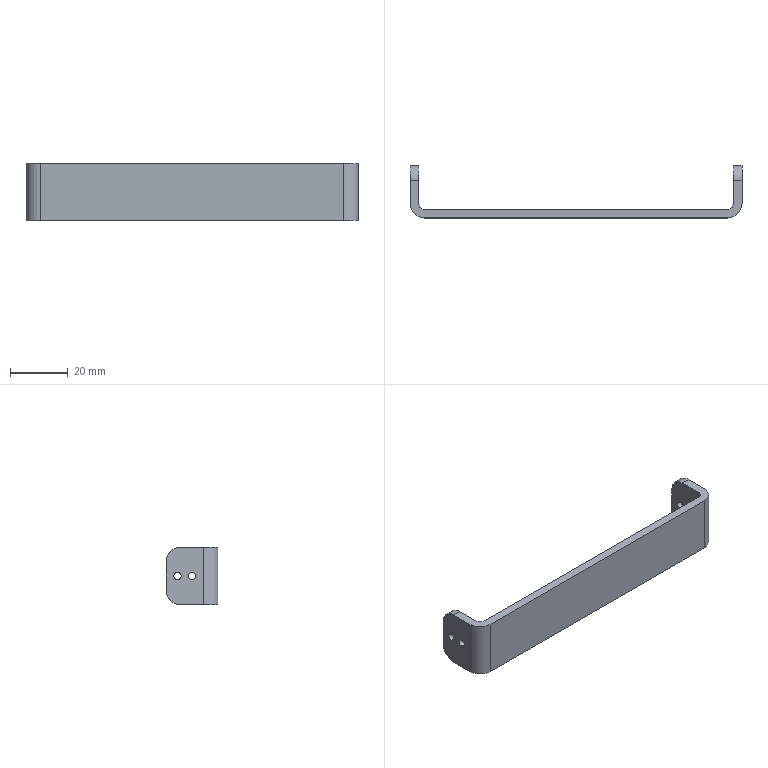Part | SolidWorks | features Fillet 3, Extrusion 1, HoleWzd 1, ICE 1 | 1 solid | 26 faces | box 115 x 18 x 20 mm | volume 8396 mm3 | cylinder 16 | plane 10 | commonest cylinder face diameters 2.5 x8 10 x6 4 x2
STEP:
#1=CARTESIAN_POINT('',(-54.5,14.,-1.25));
#2=VERTEX_POINT('',#1);
#3=CARTESIAN_POINT('',(-54.5,14.,1.25));
#4=VERTEX_POINT('',#3);
#5=CARTESIAN_POINT('',(-54.5,14.,0.));
#6=DIRECTION('',(-1.,0.,0.));
#7=DIRECTION('',(0.,0.,1.));
#8=AXIS2_PLACEMENT_3D('',#5,#6,#7);
#9=CIRCLE('',#8,1.25);
#10=EDGE_CURVE('',#2,#4,#9,.T.);
#11=ORIENTED_EDGE('',*,*,#10,.F.);
#12=CARTESIAN_POINT('',(-57.5,14.,-1.25));
#13=VERTEX_POINT('',#12);
#14=CARTESIAN_POINT('',(-57.5,14.,-1.25));
#15=DIRECTION('',(-1.,0.,0.));
#16=VECTOR('',#15,1000.);
#17=LINE('',#14,#16);
#18=EDGE_CURVE('',#2,#13,#17,.T.);
#19=ORIENTED_EDGE('',*,*,#18,.T.);
#20=CARTESIAN_POINT('',(-57.5,14.,1.25));
#21=VERTEX_POINT('',#20);
#22=CARTESIAN_POINT('',(-57.5,14.,0.));
#23=DIRECTION('',(-1.,0.,0.));
#24=DIRECTION('',(0.,0.,1.));
#25=AXIS2_PLACEMENT_3D('',#22,#23,#24);
#26=CIRCLE('',#25,1.25);
#27=EDGE_CURVE('',#13,#21,#26,.T.);
#28=ORIENTED_EDGE('',*,*,#27,.T.);
#29=CARTESIAN_POINT('',(-57.5,14.,1.25));
#30=DIRECTION('',(-1.,0.,0.));
#31=VECTOR('',#30,1000.);
#32=LINE('',#29,#31);
#33=EDGE_CURVE('',#4,#21,#32,.T.);
#34=ORIENTED_EDGE('',*,*,#33,.F.);
#35=EDGE_LOOP('',(#11,#19,#28,#34));
#36=FACE_OUTER_BOUND('',#35,.T.);
#37=CARTESIAN_POINT('',(-57.5,14.,0.));
#38=DIRECTION('',(-1.,0.,0.));
#39=DIRECTION('',(0.,0.,1.));
#40=AXIS2_PLACEMENT_3D('',#37,#38,#39);
#41=CYLINDRICAL_SURFACE('',#40,1.25);
#42=ADVANCED_FACE('',(#36),#41,.F.);
#43=CARTESIAN_POINT('',(57.5,14.,-1.25));
#44=VERTEX_POINT('',#43);
#45=CARTESIAN_POINT('',(57.5,14.,1.25));
#46=VERTEX_POINT('',#45);
#47=CARTESIAN_POINT('',(57.5,14.,0.));
#48=DIRECTION('',(-1.,0.,0.));
#49=DIRECTION('',(0.,0.,1.));
#50=AXIS2_PLACEMENT_3D('',#47,#48,#49);
#51=CIRCLE('',#50,1.25);
#52=EDGE_CURVE('',#44,#46,#51,.T.);
#53=ORIENTED_EDGE('',*,*,#52,.F.);
#54=CARTESIAN_POINT('',(54.5,14.,-1.25));
#55=VERTEX_POINT('',#54);
#56=CARTESIAN_POINT('',(-57.5,14.,-1.25));
#57=DIRECTION('',(-1.,0.,0.));
#58=VECTOR('',#57,1000.);
#59=LINE('',#56,#58);
#60=EDGE_CURVE('',#44,#55,#59,.T.);
#61=ORIENTED_EDGE('',*,*,#60,.T.);
#62=CARTESIAN_POINT('',(54.5,14.,1.25));
#63=VERTEX_POINT('',#62);
#64=CARTESIAN_POINT('',(54.5,14.,0.));
#65=DIRECTION('',(1.,0.,0.));
#66=DIRECTION('',(0.,0.,-1.));
#67=AXIS2_PLACEMENT_3D('',#64,#65,#66);
#68=CIRCLE('',#67,1.25);
#69=EDGE_CURVE('',#63,#55,#68,.T.);
#70=ORIENTED_EDGE('',*,*,#69,.F.);
#71=CARTESIAN_POINT('',(-57.5,14.,1.25));
#72=DIRECTION('',(-1.,0.,0.));
#73=VECTOR('',#72,1000.);
#74=LINE('',#71,#73);
#75=EDGE_CURVE('',#46,#63,#74,.T.);
#76=ORIENTED_EDGE('',*,*,#75,.F.);
#77=EDGE_LOOP('',(#53,#61,#70,#76));
#78=FACE_OUTER_BOUND('',#77,.T.);
#79=CARTESIAN_POINT('',(-57.5,14.,0.));
#80=DIRECTION('',(-1.,0.,0.));
#81=DIRECTION('',(0.,0.,1.));
#82=AXIS2_PLACEMENT_3D('',#79,#80,#81);
#83=CYLINDRICAL_SURFACE('',#82,1.25);
#84=ADVANCED_FACE('',(#78),#83,.F.);
#85=CARTESIAN_POINT('',(-54.5,9.,-1.25));
#86=VERTEX_POINT('',#85);
#87=CARTESIAN_POINT('',(-54.5,9.,1.25));
#88=VERTEX_POINT('',#87);
#89=CARTESIAN_POINT('',(-54.5,9.,0.));
#90=DIRECTION('',(-1.,0.,0.));
#91=DIRECTION('',(0.,0.,1.));
#92=AXIS2_PLACEMENT_3D('',#89,#90,#91);
#93=CIRCLE('',#92,1.25);
#94=EDGE_CURVE('',#86,#88,#93,.T.);
#95=ORIENTED_EDGE('',*,*,#94,.F.);
#96=CARTESIAN_POINT('',(-57.5,9.,-1.25));
#97=VERTEX_POINT('',#96);
#98=CARTESIAN_POINT('',(-57.5,9.,-1.25));
#99=DIRECTION('',(-1.,0.,0.));
#100=VECTOR('',#99,1000.);
#101=LINE('',#98,#100);
#102=EDGE_CURVE('',#86,#97,#101,.T.);
#103=ORIENTED_EDGE('',*,*,#102,.T.);
#104=CARTESIAN_POINT('',(-57.5,9.,1.25));
#105=VERTEX_POINT('',#104);
#106=CARTESIAN_POINT('',(-57.5,9.,0.));
#107=DIRECTION('',(-1.,0.,0.));
#108=DIRECTION('',(0.,0.,1.));
#109=AXIS2_PLACEMENT_3D('',#106,#107,#108);
#110=CIRCLE('',#109,1.25);
#111=EDGE_CURVE('',#97,#105,#110,.T.);
#112=ORIENTED_EDGE('',*,*,#111,.T.);
#113=CARTESIAN_POINT('',(-57.5,9.,1.25));
#114=DIRECTION('',(-1.,0.,0.));
#115=VECTOR('',#114,1000.);
#116=LINE('',#113,#115);
#117=EDGE_CURVE('',#88,#105,#116,.T.);
#118=ORIENTED_EDGE('',*,*,#117,.F.);
#119=EDGE_LOOP('',(#95,#103,#112,#118));
#120=FACE_OUTER_BOUND('',#119,.T.);
#121=CARTESIAN_POINT('',(-57.5,9.,0.));
#122=DIRECTION('',(-1.,0.,0.));
#123=DIRECTION('',(0.,0.,1.));
#124=AXIS2_PLACEMENT_3D('',#121,#122,#123);
#125=CYLINDRICAL_SURFACE('',#124,1.25);
#126=ADVANCED_FACE('',(#120),#125,.F.);
#127=CARTESIAN_POINT('',(57.5,9.,-1.25));
#128=VERTEX_POINT('',#127);
#129=CARTESIAN_POINT('',(57.5,9.,1.25));
#130=VERTEX_POINT('',#129);
#131=CARTESIAN_POINT('',(57.5,9.,0.));
#132=DIRECTION('',(-1.,0.,0.));
#133=DIRECTION('',(0.,0.,1.));
#134=AXIS2_PLACEMENT_3D('',#131,#132,#133);
#135=CIRCLE('',#134,1.25);
#136=EDGE_CURVE('',#128,#130,#135,.T.);
#137=ORIENTED_EDGE('',*,*,#136,.F.);
#138=CARTESIAN_POINT('',(54.5,9.,-1.25));
#139=VERTEX_POINT('',#138);
#140=CARTESIAN_POINT('',(-57.5,9.,-1.25));
#141=DIRECTION('',(-1.,0.,0.));
#142=VECTOR('',#141,1000.);
#143=LINE('',#140,#142);
#144=EDGE_CURVE('',#128,#139,#143,.T.);
#145=ORIENTED_EDGE('',*,*,#144,.T.);
#146=CARTESIAN_POINT('',(54.5,9.,1.25));
#147=VERTEX_POINT('',#146);
#148=CARTESIAN_POINT('',(54.5,9.,0.));
#149=DIRECTION('',(1.,0.,0.));
#150=DIRECTION('',(0.,0.,-1.));
#151=AXIS2_PLACEMENT_3D('',#148,#149,#150);
#152=CIRCLE('',#151,1.25);
#153=EDGE_CURVE('',#147,#139,#152,.T.);
#154=ORIENTED_EDGE('',*,*,#153,.F.);
#155=CARTESIAN_POINT('',(-57.5,9.,1.25));
#156=DIRECTION('',(-1.,0.,0.));
#157=VECTOR('',#156,1000.);
#158=LINE('',#155,#157);
#159=EDGE_CURVE('',#130,#147,#158,.T.);
#160=ORIENTED_EDGE('',*,*,#159,.F.);
#161=EDGE_LOOP('',(#137,#145,#154,#160));
#162=FACE_OUTER_BOUND('',#161,.T.);
#163=CARTESIAN_POINT('',(-57.5,9.,0.));
#164=DIRECTION('',(-1.,0.,0.));
#165=DIRECTION('',(0.,0.,1.));
#166=AXIS2_PLACEMENT_3D('',#163,#164,#165);
#167=CYLINDRICAL_SURFACE('',#166,1.25);
#168=ADVANCED_FACE('',(#162),#167,.F.);
#169=CARTESIAN_POINT('',(-57.5,9.,0.));
#170=DIRECTION('',(-1.,0.,0.));
#171=DIRECTION('',(0.,0.,1.));
#172=AXIS2_PLACEMENT_3D('',#169,#170,#171);
#173=CIRCLE('',#172,1.25);
#174=EDGE_CURVE('',#105,#97,#173,.T.);
#175=ORIENTED_EDGE('',*,*,#174,.F.);
#176=ORIENTED_EDGE('',*,*,#111,.F.);
#177=EDGE_LOOP('',(#175,#176));
#178=FACE_BOUND('',#177,.T.);
#179=CARTESIAN_POINT('',(-57.5,13.,10.));
#180=VERTEX_POINT('',#179);
#181=CARTESIAN_POINT('',(-57.5,5.,10.));
#182=VERTEX_POINT('',#181);
#183=CARTESIAN_POINT('',(-57.5,3.,10.));
#184=DIRECTION('',(0.,-1.,0.));
#185=VECTOR('',#184,1000.);
#186=LINE('',#183,#185);
#187=EDGE_CURVE('',#180,#182,#186,.T.);
#188=ORIENTED_EDGE('',*,*,#187,.F.);
#189=CARTESIAN_POINT('',(-57.5,18.,5.));
#190=VERTEX_POINT('',#189);
#191=CARTESIAN_POINT('',(-57.5,13.,5.));
#192=DIRECTION('',(-1.,0.,0.));
#193=DIRECTION('',(0.,0.,-1.));
#194=AXIS2_PLACEMENT_3D('',#191,#192,#193);
#195=CIRCLE('',#194,5.);
#196=EDGE_CURVE('',#180,#190,#195,.T.);
#197=ORIENTED_EDGE('',*,*,#196,.T.);
#198=CARTESIAN_POINT('',(-57.5,18.,-5.));
#199=VERTEX_POINT('',#198);
#200=CARTESIAN_POINT('',(-57.5,18.,-10.));
#201=DIRECTION('',(0.,0.,1.));
#202=VECTOR('',#201,1000.);
#203=LINE('',#200,#202);
#204=EDGE_CURVE('',#199,#190,#203,.T.);
#205=ORIENTED_EDGE('',*,*,#204,.F.);
#206=CARTESIAN_POINT('',(-57.5,13.,-10.));
#207=VERTEX_POINT('',#206);
#208=CARTESIAN_POINT('',(-57.5,13.,-5.));
#209=DIRECTION('',(-1.,0.,0.));
#210=DIRECTION('',(0.,0.,-1.));
#211=AXIS2_PLACEMENT_3D('',#208,#209,#210);
#212=CIRCLE('',#211,5.);
#213=EDGE_CURVE('',#199,#207,#212,.T.);
#214=ORIENTED_EDGE('',*,*,#213,.T.);
#215=CARTESIAN_POINT('',(-57.5,5.,-10.));
#216=VERTEX_POINT('',#215);
#217=CARTESIAN_POINT('',(-57.5,3.,-10.));
#218=DIRECTION('',(0.,-1.,0.));
#219=VECTOR('',#218,1000.);
#220=LINE('',#217,#219);
#221=EDGE_CURVE('',#207,#216,#220,.T.);
#222=ORIENTED_EDGE('',*,*,#221,.T.);
#223=CARTESIAN_POINT('',(-57.5,5.,10.));
#224=DIRECTION('',(0.,0.,1.));
#225=VECTOR('',#224,1000.);
#226=LINE('',#223,#225);
#227=EDGE_CURVE('',#216,#182,#226,.T.);
#228=ORIENTED_EDGE('',*,*,#227,.T.);
#229=EDGE_LOOP('',(#188,#197,#205,#214,#222,#228));
#230=FACE_OUTER_BOUND('',#229,.T.);
#231=CARTESIAN_POINT('',(-57.5,14.,0.));
#232=DIRECTION('',(-1.,0.,0.));
#233=DIRECTION('',(0.,0.,1.));
#234=AXIS2_PLACEMENT_3D('',#231,#232,#233);
#235=CIRCLE('',#234,1.25);
#236=EDGE_CURVE('',#21,#13,#235,.T.);
#237=ORIENTED_EDGE('',*,*,#236,.F.);
#238=ORIENTED_EDGE('',*,*,#27,.F.);
#239=EDGE_LOOP('',(#237,#238));
#240=FACE_BOUND('',#239,.T.);
#241=CARTESIAN_POINT('',(-57.5,3.,10.));
#242=DIRECTION('',(1.,0.,0.));
#243=DIRECTION('',(0.,0.,-1.));
#244=AXIS2_PLACEMENT_3D('',#241,#242,#243);
#245=PLANE('',#244);
#246=ADVANCED_FACE('',(#178,#230,#240),#245,.F.);
#247=CARTESIAN_POINT('',(-52.5,3.,10.));
#248=VERTEX_POINT('',#247);
#249=CARTESIAN_POINT('',(52.5,3.,10.));
#250=VERTEX_POINT('',#249);
#251=CARTESIAN_POINT('',(-57.5,3.,10.));
#252=DIRECTION('',(1.,0.,0.));
#253=VECTOR('',#252,1000.);
#254=LINE('',#251,#253);
#255=EDGE_CURVE('',#248,#250,#254,.T.);
#256=ORIENTED_EDGE('',*,*,#255,.T.);
#257=CARTESIAN_POINT('',(52.5,3.,-10.));
#258=VERTEX_POINT('',#257);
#259=CARTESIAN_POINT('',(52.5,3.,-10.));
#260=DIRECTION('',(0.,0.,-1.));
#261=VECTOR('',#260,1000.);
#262=LINE('',#259,#261);
#263=EDGE_CURVE('',#250,#258,#262,.T.);
#264=ORIENTED_EDGE('',*,*,#263,.T.);
#265=CARTESIAN_POINT('',(-52.5,3.,-10.));
#266=VERTEX_POINT('',#265);
#267=CARTESIAN_POINT('',(-57.5,3.,-10.));
#268=DIRECTION('',(-1.,0.,0.));
#269=VECTOR('',#268,1000.);
#270=LINE('',#267,#269);
#271=EDGE_CURVE('',#258,#266,#270,.T.);
#272=ORIENTED_EDGE('',*,*,#271,.T.);
#273=CARTESIAN_POINT('',(-52.5,3.,10.));
#274=DIRECTION('',(0.,0.,1.));
#275=VECTOR('',#274,1000.);
#276=LINE('',#273,#275);
#277=EDGE_CURVE('',#266,#248,#276,.T.);
#278=ORIENTED_EDGE('',*,*,#277,.T.);
#279=EDGE_LOOP('',(#256,#264,#272,#278));
#280=FACE_OUTER_BOUND('',#279,.T.);
#281=CARTESIAN_POINT('',(0.,3.,0.));
#282=DIRECTION('',(0.,-1.,0.));
#283=DIRECTION('',(0.,0.,-1.));
#284=AXIS2_PLACEMENT_3D('',#281,#282,#283);
#285=PLANE('',#284);
#286=ADVANCED_FACE('',(#280),#285,.F.);
#287=CARTESIAN_POINT('',(57.5,14.,0.));
#288=DIRECTION('',(-1.,0.,0.));
#289=DIRECTION('',(0.,0.,1.));
#290=AXIS2_PLACEMENT_3D('',#287,#288,#289);
#291=CIRCLE('',#290,1.25);
#292=EDGE_CURVE('',#46,#44,#291,.T.);
#293=ORIENTED_EDGE('',*,*,#292,.T.);
#294=ORIENTED_EDGE('',*,*,#52,.T.);
#295=EDGE_LOOP('',(#293,#294));
#296=FACE_BOUND('',#295,.T.);
#297=CARTESIAN_POINT('',(57.5,9.,0.));
#298=DIRECTION('',(-1.,0.,0.));
#299=DIRECTION('',(0.,0.,1.));
#300=AXIS2_PLACEMENT_3D('',#297,#298,#299);
#301=CIRCLE('',#300,1.25);
#302=EDGE_CURVE('',#130,#128,#301,.T.);
#303=ORIENTED_EDGE('',*,*,#302,.T.);
#304=ORIENTED_EDGE('',*,*,#136,.T.);
#305=EDGE_LOOP('',(#303,#304));
#306=FACE_BOUND('',#305,.T.);
#307=CARTESIAN_POINT('',(57.5,18.,5.));
#308=VERTEX_POINT('',#307);
#309=CARTESIAN_POINT('',(57.5,18.,-5.));
#310=VERTEX_POINT('',#309);
#311=CARTESIAN_POINT('',(57.5,18.,-10.));
#312=DIRECTION('',(0.,0.,-1.));
#313=VECTOR('',#312,1000.);
#314=LINE('',#311,#313);
#315=EDGE_CURVE('',#308,#310,#314,.T.);
#316=ORIENTED_EDGE('',*,*,#315,.F.);
#317=CARTESIAN_POINT('',(57.5,13.,10.));
#318=VERTEX_POINT('',#317);
#319=CARTESIAN_POINT('',(57.5,13.,5.));
#320=DIRECTION('',(1.,0.,0.));
#321=DIRECTION('',(0.,0.,1.));
#322=AXIS2_PLACEMENT_3D('',#319,#320,#321);
#323=CIRCLE('',#322,5.);
#324=EDGE_CURVE('',#308,#318,#323,.T.);
#325=ORIENTED_EDGE('',*,*,#324,.T.);
#326=CARTESIAN_POINT('',(57.5,5.,10.));
#327=VERTEX_POINT('',#326);
#328=CARTESIAN_POINT('',(57.5,3.,10.));
#329=DIRECTION('',(0.,-1.,0.));
#330=VECTOR('',#329,1000.);
#331=LINE('',#328,#330);
#332=EDGE_CURVE('',#318,#327,#331,.T.);
#333=ORIENTED_EDGE('',*,*,#332,.T.);
#334=CARTESIAN_POINT('',(57.5,5.,-10.));
#335=VERTEX_POINT('',#334);
#336=CARTESIAN_POINT('',(57.5,5.,-10.));
#337=DIRECTION('',(0.,0.,-1.));
#338=VECTOR('',#337,1000.);
#339=LINE('',#336,#338);
#340=EDGE_CURVE('',#327,#335,#339,.T.);
#341=ORIENTED_EDGE('',*,*,#340,.T.);
#342=CARTESIAN_POINT('',(57.5,13.,-10.));
#343=VERTEX_POINT('',#342);
#344=CARTESIAN_POINT('',(57.5,3.,-10.));
#345=DIRECTION('',(0.,-1.,0.));
#346=VECTOR('',#345,1000.);
#347=LINE('',#344,#346);
#348=EDGE_CURVE('',#343,#335,#347,.T.);
#349=ORIENTED_EDGE('',*,*,#348,.F.);
#350=CARTESIAN_POINT('',(57.5,13.,-5.));
#351=DIRECTION('',(1.,0.,0.));
#352=DIRECTION('',(0.,0.,1.));
#353=AXIS2_PLACEMENT_3D('',#350,#351,#352);
#354=CIRCLE('',#353,5.);
#355=EDGE_CURVE('',#343,#310,#354,.T.);
#356=ORIENTED_EDGE('',*,*,#355,.T.);
#357=EDGE_LOOP('',(#316,#325,#333,#341,#349,#356));
#358=FACE_OUTER_BOUND('',#357,.T.);
#359=CARTESIAN_POINT('',(57.5,3.,10.));
#360=DIRECTION('',(-1.,0.,0.));
#361=DIRECTION('',(0.,0.,1.));
#362=AXIS2_PLACEMENT_3D('',#359,#360,#361);
#363=PLANE('',#362);
#364=ADVANCED_FACE('',(#296,#306,#358),#363,.F.);
#365=ORIENTED_EDGE('',*,*,#221,.F.);
#366=CARTESIAN_POINT('',(-54.5,13.,-10.));
#367=VERTEX_POINT('',#366);
#368=CARTESIAN_POINT('',(-54.5,13.,-10.));
#369=DIRECTION('',(1.,0.,0.));
#370=VECTOR('',#369,1000.);
#371=LINE('',#368,#370);
#372=EDGE_CURVE('',#207,#367,#371,.T.);
#373=ORIENTED_EDGE('',*,*,#372,.T.);
#374=CARTESIAN_POINT('',(-54.5,5.,-10.));
#375=VERTEX_POINT('',#374);
#376=CARTESIAN_POINT('',(-54.5,18.,-10.));
#377=DIRECTION('',(0.,-1.,0.));
#378=VECTOR('',#377,1000.);
#379=LINE('',#376,#378);
#380=EDGE_CURVE('',#367,#375,#379,.T.);
#381=ORIENTED_EDGE('',*,*,#380,.T.);
#382=CARTESIAN_POINT('',(-52.5,5.,-10.));
#383=DIRECTION('',(0.,0.,1.));
#384=DIRECTION('',(1.,0.,0.));
#385=AXIS2_PLACEMENT_3D('',#382,#383,#384);
#386=CIRCLE('',#385,2.);
#387=EDGE_CURVE('',#375,#266,#386,.T.);
#388=ORIENTED_EDGE('',*,*,#387,.T.);
#389=ORIENTED_EDGE('',*,*,#271,.F.);
#390=CARTESIAN_POINT('',(54.5,5.,-10.));
#391=VERTEX_POINT('',#390);
#392=CARTESIAN_POINT('',(52.5,5.,-10.));
#393=DIRECTION('',(0.,0.,1.));
#394=DIRECTION('',(1.,0.,0.));
#395=AXIS2_PLACEMENT_3D('',#392,#393,#394);
#396=CIRCLE('',#395,2.);
#397=EDGE_CURVE('',#258,#391,#396,.T.);
#398=ORIENTED_EDGE('',*,*,#397,.T.);
#399=CARTESIAN_POINT('',(54.5,13.,-10.));
#400=VERTEX_POINT('',#399);
#401=CARTESIAN_POINT('',(54.5,18.,-10.));
#402=DIRECTION('',(0.,-1.,0.));
#403=VECTOR('',#402,1000.);
#404=LINE('',#401,#403);
#405=EDGE_CURVE('',#400,#391,#404,.T.);
#406=ORIENTED_EDGE('',*,*,#405,.F.);
#407=CARTESIAN_POINT('',(-57.5,13.,-10.));
#408=DIRECTION('',(1.,0.,0.));
#409=VECTOR('',#408,1000.);
#410=LINE('',#407,#409);
#411=EDGE_CURVE('',#400,#343,#410,.T.);
#412=ORIENTED_EDGE('',*,*,#411,.T.);
#413=ORIENTED_EDGE('',*,*,#348,.T.);
#414=CARTESIAN_POINT('',(52.5,0.,-10.));
#415=VERTEX_POINT('',#414);
#416=CARTESIAN_POINT('',(52.5,5.,-10.));
#417=DIRECTION('',(0.,0.,-1.));
#418=DIRECTION('',(1.,0.,0.));
#419=AXIS2_PLACEMENT_3D('',#416,#417,#418);
#420=CIRCLE('',#419,5.);
#421=EDGE_CURVE('',#335,#415,#420,.T.);
#422=ORIENTED_EDGE('',*,*,#421,.T.);
#423=CARTESIAN_POINT('',(-52.5,0.,-10.));
#424=VERTEX_POINT('',#423);
#425=CARTESIAN_POINT('',(-57.5,0.,-10.));
#426=DIRECTION('',(-1.,0.,0.));
#427=VECTOR('',#426,1000.);
#428=LINE('',#425,#427);
#429=EDGE_CURVE('',#415,#424,#428,.T.);
#430=ORIENTED_EDGE('',*,*,#429,.T.);
#431=CARTESIAN_POINT('',(-52.5,5.,-10.));
#432=DIRECTION('',(0.,0.,-1.));
#433=DIRECTION('',(1.,0.,0.));
#434=AXIS2_PLACEMENT_3D('',#431,#432,#433);
#435=CIRCLE('',#434,5.);
#436=EDGE_CURVE('',#424,#216,#435,.T.);
#437=ORIENTED_EDGE('',*,*,#436,.T.);
#438=EDGE_LOOP('',(#365,#373,#381,#388,#389,#398,#406,#412,#413,#422,#430,#437));
#439=FACE_OUTER_BOUND('',#438,.T.);
#440=CARTESIAN_POINT('',(-57.5,3.,-10.));
#441=DIRECTION('',(0.,0.,1.));
#442=DIRECTION('',(1.,0.,0.));
#443=AXIS2_PLACEMENT_3D('',#440,#441,#442);
#444=PLANE('',#443);
#445=ADVANCED_FACE('',(#439),#444,.F.);
#446=CARTESIAN_POINT('',(-54.5,13.,10.));
#447=VERTEX_POINT('',#446);
#448=CARTESIAN_POINT('',(-54.5,5.,10.));
#449=VERTEX_POINT('',#448);
#450=CARTESIAN_POINT('',(-54.5,18.,10.));
#451=DIRECTION('',(0.,-1.,0.));
#452=VECTOR('',#451,1000.);
#453=LINE('',#450,#452);
#454=EDGE_CURVE('',#447,#449,#453,.T.);
#455=ORIENTED_EDGE('',*,*,#454,.F.);
#456=CARTESIAN_POINT('',(-57.5,13.,10.));
#457=DIRECTION('',(-1.,0.,0.));
#458=VECTOR('',#457,1000.);
#459=LINE('',#456,#458);
#460=EDGE_CURVE('',#447,#180,#459,.T.);
#461=ORIENTED_EDGE('',*,*,#460,.T.);
#462=ORIENTED_EDGE('',*,*,#187,.T.);
#463=CARTESIAN_POINT('',(-52.5,0.,10.));
#464=VERTEX_POINT('',#463);
#465=CARTESIAN_POINT('',(-52.5,5.,10.));
#466=DIRECTION('',(0.,0.,1.));
#467=DIRECTION('',(-1.,0.,0.));
#468=AXIS2_PLACEMENT_3D('',#465,#466,#467);
#469=CIRCLE('',#468,5.);
#470=EDGE_CURVE('',#182,#464,#469,.T.);
#471=ORIENTED_EDGE('',*,*,#470,.T.);
#472=CARTESIAN_POINT('',(52.5,0.,10.));
#473=VERTEX_POINT('',#472);
#474=CARTESIAN_POINT('',(-57.5,0.,10.));
#475=DIRECTION('',(1.,0.,0.));
#476=VECTOR('',#475,1000.);
#477=LINE('',#474,#476);
#478=EDGE_CURVE('',#464,#473,#477,.T.);
#479=ORIENTED_EDGE('',*,*,#478,.T.);
#480=CARTESIAN_POINT('',(52.5,5.,10.));
#481=DIRECTION('',(0.,0.,1.));
#482=DIRECTION('',(-1.,0.,0.));
#483=AXIS2_PLACEMENT_3D('',#480,#481,#482);
#484=CIRCLE('',#483,5.);
#485=EDGE_CURVE('',#473,#327,#484,.T.);
#486=ORIENTED_EDGE('',*,*,#485,.T.);
#487=ORIENTED_EDGE('',*,*,#332,.F.);
#488=CARTESIAN_POINT('',(54.5,13.,10.));
#489=VERTEX_POINT('',#488);
#490=CARTESIAN_POINT('',(-57.5,13.,10.));
#491=DIRECTION('',(-1.,0.,0.));
#492=VECTOR('',#491,1000.);
#493=LINE('',#490,#492);
#494=EDGE_CURVE('',#318,#489,#493,.T.);
#495=ORIENTED_EDGE('',*,*,#494,.T.);
#496=CARTESIAN_POINT('',(54.5,5.,10.));
#497=VERTEX_POINT('',#496);
#498=CARTESIAN_POINT('',(54.5,18.,10.));
#499=DIRECTION('',(0.,-1.,0.));
#500=VECTOR('',#499,1000.);
#501=LINE('',#498,#500);
#502=EDGE_CURVE('',#489,#497,#501,.T.);
#503=ORIENTED_EDGE('',*,*,#502,.T.);
#504=CARTESIAN_POINT('',(52.5,5.,10.));
#505=DIRECTION('',(0.,0.,-1.));
#506=DIRECTION('',(-1.,0.,0.));
#507=AXIS2_PLACEMENT_3D('',#504,#505,#506);
#508=CIRCLE('',#507,2.);
#509=EDGE_CURVE('',#497,#250,#508,.T.);
#510=ORIENTED_EDGE('',*,*,#509,.T.);
#511=ORIENTED_EDGE('',*,*,#255,.F.);
#512=CARTESIAN_POINT('',(-52.5,5.,10.));
#513=DIRECTION('',(0.,0.,-1.));
#514=DIRECTION('',(-1.,0.,0.));
#515=AXIS2_PLACEMENT_3D('',#512,#513,#514);
#516=CIRCLE('',#515,2.);
#517=EDGE_CURVE('',#248,#449,#516,.T.);
#518=ORIENTED_EDGE('',*,*,#517,.T.);
#519=EDGE_LOOP('',(#455,#461,#462,#471,#479,#486,#487,#495,#503,#510,#511,#518));
#520=FACE_OUTER_BOUND('',#519,.T.);
#521=CARTESIAN_POINT('',(-57.5,3.,10.));
#522=DIRECTION('',(0.,0.,-1.));
#523=DIRECTION('',(-1.,0.,0.));
#524=AXIS2_PLACEMENT_3D('',#521,#522,#523);
#525=PLANE('',#524);
#526=ADVANCED_FACE('',(#520),#525,.F.);
#527=ORIENTED_EDGE('',*,*,#429,.F.);
#528=CARTESIAN_POINT('',(52.5,0.,10.));
#529=DIRECTION('',(0.,0.,1.));
#530=VECTOR('',#529,1000.);
#531=LINE('',#528,#530);
#532=EDGE_CURVE('',#415,#473,#531,.T.);
#533=ORIENTED_EDGE('',*,*,#532,.T.);
#534=ORIENTED_EDGE('',*,*,#478,.F.);
#535=CARTESIAN_POINT('',(-52.5,0.,-10.));
#536=DIRECTION('',(0.,0.,-1.));
#537=VECTOR('',#536,1000.);
#538=LINE('',#535,#537);
#539=EDGE_CURVE('',#464,#424,#538,.T.);
#540=ORIENTED_EDGE('',*,*,#539,.T.);
#541=EDGE_LOOP('',(#527,#533,#534,#540));
#542=FACE_OUTER_BOUND('',#541,.T.);
#543=CARTESIAN_POINT('',(0.,0.,0.));
#544=DIRECTION('',(0.,-1.,0.));
#545=DIRECTION('',(0.,0.,-1.));
#546=AXIS2_PLACEMENT_3D('',#543,#544,#545);
#547=PLANE('',#546);
#548=ADVANCED_FACE('',(#542),#547,.T.);
#549=CARTESIAN_POINT('',(-54.5,14.,0.));
#550=DIRECTION('',(-1.,0.,0.));
#551=DIRECTION('',(0.,0.,1.));
#552=AXIS2_PLACEMENT_3D('',#549,#550,#551);
#553=CIRCLE('',#552,1.25);
#554=EDGE_CURVE('',#4,#2,#553,.T.);
#555=ORIENTED_EDGE('',*,*,#554,.T.);
#556=ORIENTED_EDGE('',*,*,#10,.T.);
#557=EDGE_LOOP('',(#555,#556));
#558=FACE_BOUND('',#557,.T.);
#559=CARTESIAN_POINT('',(-54.5,9.,0.));
#560=DIRECTION('',(-1.,0.,0.));
#561=DIRECTION('',(0.,0.,1.));
#562=AXIS2_PLACEMENT_3D('',#559,#560,#561);
#563=CIRCLE('',#562,1.25);
#564=EDGE_CURVE('',#88,#86,#563,.T.);
#565=ORIENTED_EDGE('',*,*,#564,.T.);
#566=ORIENTED_EDGE('',*,*,#94,.T.);
#567=EDGE_LOOP('',(#565,#566));
#568=FACE_BOUND('',#567,.T.);
#569=CARTESIAN_POINT('',(-54.5,18.,5.));
#570=VERTEX_POINT('',#569);
#571=CARTESIAN_POINT('',(-54.5,18.,-5.));
#572=VERTEX_POINT('',#571);
#573=CARTESIAN_POINT('',(-54.5,18.,-10.));
#574=DIRECTION('',(0.,0.,-1.));
#575=VECTOR('',#574,1000.);
#576=LINE('',#573,#575);
#577=EDGE_CURVE('',#570,#572,#576,.T.);
#578=ORIENTED_EDGE('',*,*,#577,.F.);
#579=CARTESIAN_POINT('',(-54.5,13.,5.));
#580=DIRECTION('',(1.,0.,0.));
#581=DIRECTION('',(0.,0.,1.));
#582=AXIS2_PLACEMENT_3D('',#579,#580,#581);
#583=CIRCLE('',#582,5.);
#584=EDGE_CURVE('',#570,#447,#583,.T.);
#585=ORIENTED_EDGE('',*,*,#584,.T.);
#586=ORIENTED_EDGE('',*,*,#454,.T.);
#587=CARTESIAN_POINT('',(-54.5,5.,-10.));
#588=DIRECTION('',(0.,0.,-1.));
#589=VECTOR('',#588,1000.);
#590=LINE('',#587,#589);
#591=EDGE_CURVE('',#449,#375,#590,.T.);
#592=ORIENTED_EDGE('',*,*,#591,.T.);
#593=ORIENTED_EDGE('',*,*,#380,.F.);
#594=CARTESIAN_POINT('',(-54.5,13.,-5.));
#595=DIRECTION('',(1.,0.,0.));
#596=DIRECTION('',(0.,0.,1.));
#597=AXIS2_PLACEMENT_3D('',#594,#595,#596);
#598=CIRCLE('',#597,5.);
#599=EDGE_CURVE('',#367,#572,#598,.T.);
#600=ORIENTED_EDGE('',*,*,#599,.T.);
#601=EDGE_LOOP('',(#578,#585,#586,#592,#593,#600));
#602=FACE_OUTER_BOUND('',#601,.T.);
#603=CARTESIAN_POINT('',(-54.5,18.,-10.));
#604=DIRECTION('',(-1.,0.,0.));
#605=DIRECTION('',(0.,0.,1.));
#606=AXIS2_PLACEMENT_3D('',#603,#604,#605);
#607=PLANE('',#606);
#608=ADVANCED_FACE('',(#558,#568,#602),#607,.F.);
#609=ORIENTED_EDGE('',*,*,#204,.T.);
#610=CARTESIAN_POINT('',(-54.5,18.,5.));
#611=DIRECTION('',(1.,0.,0.));
#612=VECTOR('',#611,1000.);
#613=LINE('',#610,#612);
#614=EDGE_CURVE('',#190,#570,#613,.T.);
#615=ORIENTED_EDGE('',*,*,#614,.T.);
#616=ORIENTED_EDGE('',*,*,#577,.T.);
#617=CARTESIAN_POINT('',(-57.5,18.,-5.));
#618=DIRECTION('',(-1.,0.,0.));
#619=VECTOR('',#618,1000.);
#620=LINE('',#617,#619);
#621=EDGE_CURVE('',#572,#199,#620,.T.);
#622=ORIENTED_EDGE('',*,*,#621,.T.);
#623=EDGE_LOOP('',(#609,#615,#616,#622));
#624=FACE_OUTER_BOUND('',#623,.T.);
#625=CARTESIAN_POINT('',(0.,18.,0.));
#626=DIRECTION('',(0.,1.,0.));
#627=DIRECTION('',(0.,0.,1.));
#628=AXIS2_PLACEMENT_3D('',#625,#626,#627);
#629=PLANE('',#628);
#630=ADVANCED_FACE('',(#624),#629,.T.);
#631=ORIENTED_EDGE('',*,*,#69,.T.);
#632=CARTESIAN_POINT('',(54.5,14.,0.));
#633=DIRECTION('',(1.,0.,0.));
#634=DIRECTION('',(0.,0.,-1.));
#635=AXIS2_PLACEMENT_3D('',#632,#633,#634);
#636=CIRCLE('',#635,1.25);
#637=EDGE_CURVE('',#55,#63,#636,.T.);
#638=ORIENTED_EDGE('',*,*,#637,.T.);
#639=EDGE_LOOP('',(#631,#638));
#640=FACE_BOUND('',#639,.T.);
#641=ORIENTED_EDGE('',*,*,#153,.T.);
#642=CARTESIAN_POINT('',(54.5,9.,0.));
#643=DIRECTION('',(1.,0.,0.));
#644=DIRECTION('',(0.,0.,-1.));
#645=AXIS2_PLACEMENT_3D('',#642,#643,#644);
#646=CIRCLE('',#645,1.25);
#647=EDGE_CURVE('',#139,#147,#646,.T.);
#648=ORIENTED_EDGE('',*,*,#647,.T.);
#649=EDGE_LOOP('',(#641,#648));
#650=FACE_BOUND('',#649,.T.);
#651=ORIENTED_EDGE('',*,*,#502,.F.);
#652=CARTESIAN_POINT('',(54.5,18.,5.));
#653=VERTEX_POINT('',#652);
#654=CARTESIAN_POINT('',(54.5,13.,5.));
#655=DIRECTION('',(-1.,0.,0.));
#656=DIRECTION('',(0.,0.,-1.));
#657=AXIS2_PLACEMENT_3D('',#654,#655,#656);
#658=CIRCLE('',#657,5.);
#659=EDGE_CURVE('',#489,#653,#658,.T.);
#660=ORIENTED_EDGE('',*,*,#659,.T.);
#661=CARTESIAN_POINT('',(54.5,18.,-5.));
#662=VERTEX_POINT('',#661);
#663=CARTESIAN_POINT('',(54.5,18.,-10.));
#664=DIRECTION('',(0.,0.,1.));
#665=VECTOR('',#664,1000.);
#666=LINE('',#663,#665);
#667=EDGE_CURVE('',#662,#653,#666,.T.);
#668=ORIENTED_EDGE('',*,*,#667,.F.);
#669=CARTESIAN_POINT('',(54.5,13.,-5.));
#670=DIRECTION('',(-1.,0.,0.));
#671=DIRECTION('',(0.,0.,-1.));
#672=AXIS2_PLACEMENT_3D('',#669,#670,#671);
#673=CIRCLE('',#672,5.);
#674=EDGE_CURVE('',#662,#400,#673,.T.);
#675=ORIENTED_EDGE('',*,*,#674,.T.);
#676=ORIENTED_EDGE('',*,*,#405,.T.);
#677=CARTESIAN_POINT('',(54.5,5.,10.));
#678=DIRECTION('',(0.,0.,1.));
#679=VECTOR('',#678,1000.);
#680=LINE('',#677,#679);
#681=EDGE_CURVE('',#391,#497,#680,.T.);
#682=ORIENTED_EDGE('',*,*,#681,.T.);
#683=EDGE_LOOP('',(#651,#660,#668,#675,#676,#682));
#684=FACE_OUTER_BOUND('',#683,.T.);
#685=CARTESIAN_POINT('',(54.5,18.,-10.));
#686=DIRECTION('',(1.,0.,0.));
#687=DIRECTION('',(0.,0.,-1.));
#688=AXIS2_PLACEMENT_3D('',#685,#686,#687);
#689=PLANE('',#688);
#690=ADVANCED_FACE('',(#640,#650,#684),#689,.F.);
#691=ORIENTED_EDGE('',*,*,#667,.T.);
#692=CARTESIAN_POINT('',(0.,18.,5.));
#693=DIRECTION('',(1.,0.,0.));
#694=VECTOR('',#693,1000.);
#695=LINE('',#692,#694);
#696=EDGE_CURVE('',#653,#308,#695,.T.);
#697=ORIENTED_EDGE('',*,*,#696,.T.);
#698=ORIENTED_EDGE('',*,*,#315,.T.);
#699=CARTESIAN_POINT('',(0.,18.,-5.));
#700=DIRECTION('',(-1.,0.,0.));
#701=VECTOR('',#700,1000.);
#702=LINE('',#699,#701);
#703=EDGE_CURVE('',#310,#662,#702,.T.);
#704=ORIENTED_EDGE('',*,*,#703,.T.);
#705=EDGE_LOOP('',(#691,#697,#698,#704));
#706=FACE_OUTER_BOUND('',#705,.T.);
#707=CARTESIAN_POINT('',(0.,18.,0.));
#708=DIRECTION('',(0.,-1.,0.));
#709=DIRECTION('',(0.,0.,-1.));
#710=AXIS2_PLACEMENT_3D('',#707,#708,#709);
#711=PLANE('',#710);
#712=ADVANCED_FACE('',(#706),#711,.F.);
#713=ORIENTED_EDGE('',*,*,#397,.F.);
#714=ORIENTED_EDGE('',*,*,#263,.F.);
#715=ORIENTED_EDGE('',*,*,#509,.F.);
#716=ORIENTED_EDGE('',*,*,#681,.F.);
#717=EDGE_LOOP('',(#713,#714,#715,#716));
#718=FACE_OUTER_BOUND('',#717,.T.);
#719=CARTESIAN_POINT('',(52.5,5.,-10.));
#720=DIRECTION('',(0.,0.,-1.));
#721=DIRECTION('',(-1.,0.,0.));
#722=AXIS2_PLACEMENT_3D('',#719,#720,#721);
#723=CYLINDRICAL_SURFACE('',#722,2.);
#724=ADVANCED_FACE('',(#718),#723,.F.);
#725=ORIENTED_EDGE('',*,*,#517,.F.);
#726=ORIENTED_EDGE('',*,*,#277,.F.);
#727=ORIENTED_EDGE('',*,*,#387,.F.);
#728=ORIENTED_EDGE('',*,*,#591,.F.);
#729=EDGE_LOOP('',(#725,#726,#727,#728));
#730=FACE_OUTER_BOUND('',#729,.T.);
#731=CARTESIAN_POINT('',(-52.5,5.,-10.));
#732=DIRECTION('',(0.,0.,1.));
#733=DIRECTION('',(1.,0.,0.));
#734=AXIS2_PLACEMENT_3D('',#731,#732,#733);
#735=CYLINDRICAL_SURFACE('',#734,2.);
#736=ADVANCED_FACE('',(#730),#735,.F.);
#737=ORIENTED_EDGE('',*,*,#485,.F.);
#738=ORIENTED_EDGE('',*,*,#532,.F.);
#739=ORIENTED_EDGE('',*,*,#421,.F.);
#740=ORIENTED_EDGE('',*,*,#340,.F.);
#741=EDGE_LOOP('',(#737,#738,#739,#740));
#742=FACE_OUTER_BOUND('',#741,.T.);
#743=CARTESIAN_POINT('',(52.5,5.,10.));
#744=DIRECTION('',(0.,0.,1.));
#745=DIRECTION('',(1.,0.,0.));
#746=AXIS2_PLACEMENT_3D('',#743,#744,#745);
#747=CYLINDRICAL_SURFACE('',#746,5.);
#748=ADVANCED_FACE('',(#742),#747,.T.);
#749=ORIENTED_EDGE('',*,*,#436,.F.);
#750=ORIENTED_EDGE('',*,*,#539,.F.);
#751=ORIENTED_EDGE('',*,*,#470,.F.);
#752=ORIENTED_EDGE('',*,*,#227,.F.);
#753=EDGE_LOOP('',(#749,#750,#751,#752));
#754=FACE_OUTER_BOUND('',#753,.T.);
#755=CARTESIAN_POINT('',(-52.5,5.,10.));
#756=DIRECTION('',(0.,0.,-1.));
#757=DIRECTION('',(-1.,0.,0.));
#758=AXIS2_PLACEMENT_3D('',#755,#756,#757);
#759=CYLINDRICAL_SURFACE('',#758,5.);
#760=ADVANCED_FACE('',(#754),#759,.T.);
#761=ORIENTED_EDGE('',*,*,#144,.F.);
#762=ORIENTED_EDGE('',*,*,#302,.F.);
#763=ORIENTED_EDGE('',*,*,#159,.T.);
#764=ORIENTED_EDGE('',*,*,#647,.F.);
#765=EDGE_LOOP('',(#761,#762,#763,#764));
#766=FACE_OUTER_BOUND('',#765,.T.);
#767=CARTESIAN_POINT('',(-57.5,9.,0.));
#768=DIRECTION('',(-1.,0.,0.));
#769=DIRECTION('',(0.,0.,1.));
#770=AXIS2_PLACEMENT_3D('',#767,#768,#769);
#771=CYLINDRICAL_SURFACE('',#770,1.25);
#772=ADVANCED_FACE('',(#766),#771,.F.);
#773=ORIENTED_EDGE('',*,*,#102,.F.);
#774=ORIENTED_EDGE('',*,*,#564,.F.);
#775=ORIENTED_EDGE('',*,*,#117,.T.);
#776=ORIENTED_EDGE('',*,*,#174,.T.);
#777=EDGE_LOOP('',(#773,#774,#775,#776));
#778=FACE_OUTER_BOUND('',#777,.T.);
#779=CARTESIAN_POINT('',(-57.5,9.,0.));
#780=DIRECTION('',(-1.,0.,0.));
#781=DIRECTION('',(0.,0.,1.));
#782=AXIS2_PLACEMENT_3D('',#779,#780,#781);
#783=CYLINDRICAL_SURFACE('',#782,1.25);
#784=ADVANCED_FACE('',(#778),#783,.F.);
#785=ORIENTED_EDGE('',*,*,#60,.F.);
#786=ORIENTED_EDGE('',*,*,#292,.F.);
#787=ORIENTED_EDGE('',*,*,#75,.T.);
#788=ORIENTED_EDGE('',*,*,#637,.F.);
#789=EDGE_LOOP('',(#785,#786,#787,#788));
#790=FACE_OUTER_BOUND('',#789,.T.);
#791=CARTESIAN_POINT('',(-57.5,14.,0.));
#792=DIRECTION('',(-1.,0.,0.));
#793=DIRECTION('',(0.,0.,1.));
#794=AXIS2_PLACEMENT_3D('',#791,#792,#793);
#795=CYLINDRICAL_SURFACE('',#794,1.25);
#796=ADVANCED_FACE('',(#790),#795,.F.);
#797=ORIENTED_EDGE('',*,*,#18,.F.);
#798=ORIENTED_EDGE('',*,*,#554,.F.);
#799=ORIENTED_EDGE('',*,*,#33,.T.);
#800=ORIENTED_EDGE('',*,*,#236,.T.);
#801=EDGE_LOOP('',(#797,#798,#799,#800));
#802=FACE_OUTER_BOUND('',#801,.T.);
#803=CARTESIAN_POINT('',(-57.5,14.,0.));
#804=DIRECTION('',(-1.,0.,0.));
#805=DIRECTION('',(0.,0.,1.));
#806=AXIS2_PLACEMENT_3D('',#803,#804,#805);
#807=CYLINDRICAL_SURFACE('',#806,1.25);
#808=ADVANCED_FACE('',(#802),#807,.F.);
#809=ORIENTED_EDGE('',*,*,#196,.F.);
#810=ORIENTED_EDGE('',*,*,#460,.F.);
#811=ORIENTED_EDGE('',*,*,#584,.F.);
#812=ORIENTED_EDGE('',*,*,#614,.F.);
#813=EDGE_LOOP('',(#809,#810,#811,#812));
#814=FACE_OUTER_BOUND('',#813,.T.);
#815=CARTESIAN_POINT('',(0.,13.,5.));
#816=DIRECTION('',(-1.,0.,0.));
#817=DIRECTION('',(0.,0.,1.));
#818=AXIS2_PLACEMENT_3D('',#815,#816,#817);
#819=CYLINDRICAL_SURFACE('',#818,5.);
#820=ADVANCED_FACE('',(#814),#819,.T.);
#821=ORIENTED_EDGE('',*,*,#599,.F.);
#822=ORIENTED_EDGE('',*,*,#372,.F.);
#823=ORIENTED_EDGE('',*,*,#213,.F.);
#824=ORIENTED_EDGE('',*,*,#621,.F.);
#825=EDGE_LOOP('',(#821,#822,#823,#824));
#826=FACE_OUTER_BOUND('',#825,.T.);
#827=CARTESIAN_POINT('',(0.,13.,-5.));
#828=DIRECTION('',(1.,0.,0.));
#829=DIRECTION('',(0.,0.,-1.));
#830=AXIS2_PLACEMENT_3D('',#827,#828,#829);
#831=CYLINDRICAL_SURFACE('',#830,5.);
#832=ADVANCED_FACE('',(#826),#831,.T.);
#833=ORIENTED_EDGE('',*,*,#659,.F.);
#834=ORIENTED_EDGE('',*,*,#494,.F.);
#835=ORIENTED_EDGE('',*,*,#324,.F.);
#836=ORIENTED_EDGE('',*,*,#696,.F.);
#837=EDGE_LOOP('',(#833,#834,#835,#836));
#838=FACE_OUTER_BOUND('',#837,.T.);
#839=CARTESIAN_POINT('',(0.,13.,5.));
#840=DIRECTION('',(1.,0.,0.));
#841=DIRECTION('',(0.,0.,-1.));
#842=AXIS2_PLACEMENT_3D('',#839,#840,#841);
#843=CYLINDRICAL_SURFACE('',#842,5.);
#844=ADVANCED_FACE('',(#838),#843,.T.);
#845=ORIENTED_EDGE('',*,*,#355,.F.);
#846=ORIENTED_EDGE('',*,*,#411,.F.);
#847=ORIENTED_EDGE('',*,*,#674,.F.);
#848=ORIENTED_EDGE('',*,*,#703,.F.);
#849=EDGE_LOOP('',(#845,#846,#847,#848));
#850=FACE_OUTER_BOUND('',#849,.T.);
#851=CARTESIAN_POINT('',(0.,13.,-5.));
#852=DIRECTION('',(-1.,0.,0.));
#853=DIRECTION('',(0.,0.,1.));
#854=AXIS2_PLACEMENT_3D('',#851,#852,#853);
#855=CYLINDRICAL_SURFACE('',#854,5.);
#856=ADVANCED_FACE('',(#850),#855,.T.);
#857=CLOSED_SHELL('',(#42,#84,#126,#168,#246,#286,#364,#445,#526,#548,#608,#630,#690,#712,#724,#736,#748,#760,#772,#784,#796,#808,#820,#832,#844,#856));
#858=MANIFOLD_SOLID_BREP('',#857);
#859=CARTESIAN_POINT('',(0.,0.,0.));
#860=DIRECTION('',(0.,0.,1.));
#861=DIRECTION('',(1.,0.,0.));
#862=AXIS2_PLACEMENT_3D('',#859,#860,#861);
#863=(LENGTH_UNIT()NAMED_UNIT(*)SI_UNIT(.MILLI.,.METRE.));
#864=UNCERTAINTY_MEASURE_WITH_UNIT(LENGTH_MEASURE(0.00001),#863,'','');
#865=(NAMED_UNIT(*)PLANE_ANGLE_UNIT()SI_UNIT($,.RADIAN.));
#866=(NAMED_UNIT(*)SI_UNIT($,.STERADIAN.)SOLID_ANGLE_UNIT());
#867=(GEOMETRIC_REPRESENTATION_CONTEXT(3)GLOBAL_UNCERTAINTY_ASSIGNED_CONTEXT((#864))GLOBAL_UNIT_ASSIGNED_CONTEXT((#863,#865,#866))REPRESENTATION_CONTEXT('',''));
#868=ADVANCED_BREP_SHAPE_REPRESENTATION('',(#858,#862),#867);